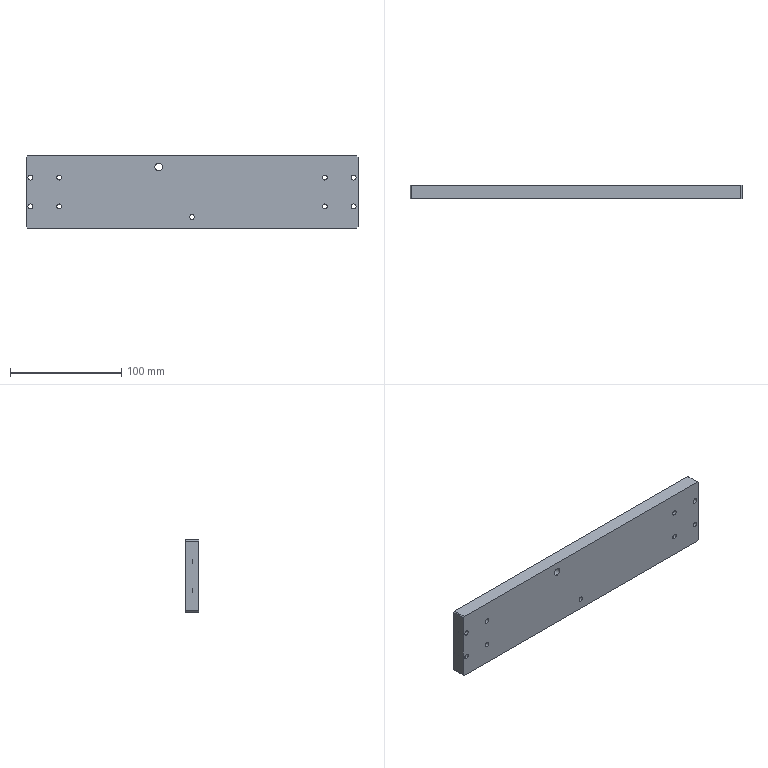Part | STEP file | A14-024 | 1 solid | 58 faces | box 299 x 12 x 65 mm | volume 229704 mm3 | cylinder 36 | plane 18 | cone 4 | commonest cylinder face diameters 4.5 x16 7.5 x16 4.2 x2 6.8 x2